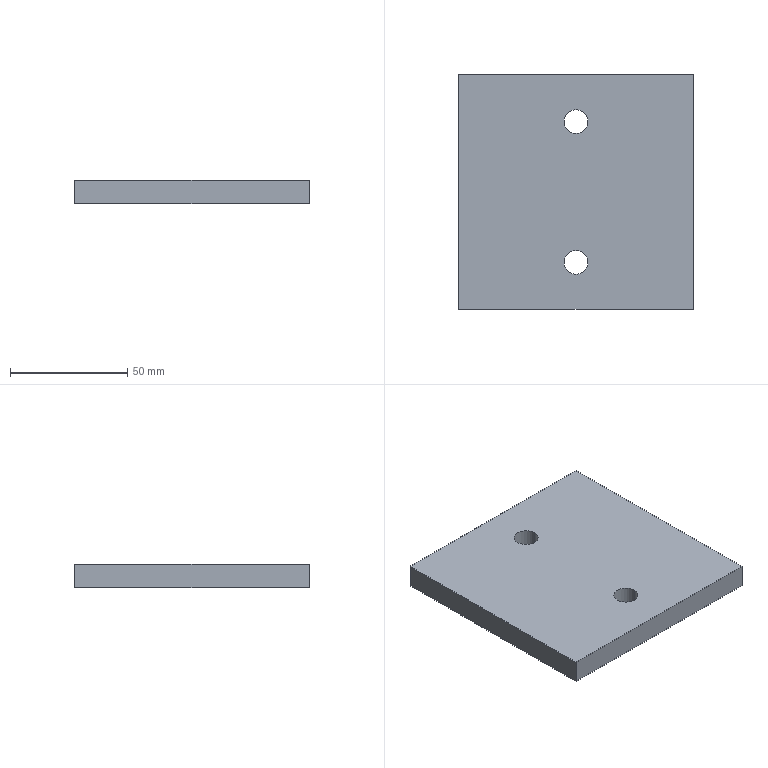Part | SolidWorks | features Extrusion 1, HoleWzd 1 | 1 solid | 10 faces | box 100 x 100 x 10 mm | volume 98366 mm3 | plane 6 | cylinder 4 | commonest cylinder face diameters 10.2 x4
STEP:
#1=CARTESIAN_POINT('',(5.1,30.,0.));
#2=VERTEX_POINT('',#1);
#3=CARTESIAN_POINT('',(-5.1,30.,0.));
#4=VERTEX_POINT('',#3);
#5=CARTESIAN_POINT('',(0.,30.,0.));
#6=DIRECTION('',(0.,0.,-1.));
#7=DIRECTION('',(-1.,0.,0.));
#8=AXIS2_PLACEMENT_3D('',#5,#6,#7);
#9=CIRCLE('',#8,5.1);
#10=EDGE_CURVE('',#2,#4,#9,.T.);
#11=ORIENTED_EDGE('',*,*,#10,.T.);
#12=CARTESIAN_POINT('',(-5.1,30.,10.));
#13=VERTEX_POINT('',#12);
#14=CARTESIAN_POINT('',(-5.1,30.,10.));
#15=DIRECTION('',(0.,0.,1.));
#16=VECTOR('',#15,1000.);
#17=LINE('',#14,#16);
#18=EDGE_CURVE('',#4,#13,#17,.T.);
#19=ORIENTED_EDGE('',*,*,#18,.T.);
#20=CARTESIAN_POINT('',(5.1,30.,10.));
#21=VERTEX_POINT('',#20);
#22=CARTESIAN_POINT('',(0.,30.,10.));
#23=DIRECTION('',(0.,0.,1.));
#24=DIRECTION('',(1.,0.,0.));
#25=AXIS2_PLACEMENT_3D('',#22,#23,#24);
#26=CIRCLE('',#25,5.1);
#27=EDGE_CURVE('',#13,#21,#26,.T.);
#28=ORIENTED_EDGE('',*,*,#27,.T.);
#29=CARTESIAN_POINT('',(5.1,30.,10.));
#30=DIRECTION('',(0.,0.,1.));
#31=VECTOR('',#30,1000.);
#32=LINE('',#29,#31);
#33=EDGE_CURVE('',#2,#21,#32,.T.);
#34=ORIENTED_EDGE('',*,*,#33,.F.);
#35=EDGE_LOOP('',(#11,#19,#28,#34));
#36=FACE_OUTER_BOUND('',#35,.T.);
#37=CARTESIAN_POINT('',(0.,30.,10.));
#38=DIRECTION('',(0.,0.,1.));
#39=DIRECTION('',(1.,0.,0.));
#40=AXIS2_PLACEMENT_3D('',#37,#38,#39);
#41=CYLINDRICAL_SURFACE('',#40,5.1);
#42=ADVANCED_FACE('',(#36),#41,.F.);
#43=CARTESIAN_POINT('',(5.1,-30.,0.));
#44=VERTEX_POINT('',#43);
#45=CARTESIAN_POINT('',(-5.1,-30.,0.));
#46=VERTEX_POINT('',#45);
#47=CARTESIAN_POINT('',(0.,-30.,0.));
#48=DIRECTION('',(0.,0.,-1.));
#49=DIRECTION('',(-1.,0.,0.));
#50=AXIS2_PLACEMENT_3D('',#47,#48,#49);
#51=CIRCLE('',#50,5.1);
#52=EDGE_CURVE('',#44,#46,#51,.T.);
#53=ORIENTED_EDGE('',*,*,#52,.T.);
#54=CARTESIAN_POINT('',(-5.1,-30.,10.));
#55=VERTEX_POINT('',#54);
#56=CARTESIAN_POINT('',(-5.1,-30.,10.));
#57=DIRECTION('',(0.,0.,1.));
#58=VECTOR('',#57,1000.);
#59=LINE('',#56,#58);
#60=EDGE_CURVE('',#46,#55,#59,.T.);
#61=ORIENTED_EDGE('',*,*,#60,.T.);
#62=CARTESIAN_POINT('',(5.1,-30.,10.));
#63=VERTEX_POINT('',#62);
#64=CARTESIAN_POINT('',(0.,-30.,10.));
#65=DIRECTION('',(0.,0.,1.));
#66=DIRECTION('',(1.,0.,0.));
#67=AXIS2_PLACEMENT_3D('',#64,#65,#66);
#68=CIRCLE('',#67,5.1);
#69=EDGE_CURVE('',#55,#63,#68,.T.);
#70=ORIENTED_EDGE('',*,*,#69,.T.);
#71=CARTESIAN_POINT('',(5.1,-30.,10.));
#72=DIRECTION('',(0.,0.,1.));
#73=VECTOR('',#72,1000.);
#74=LINE('',#71,#73);
#75=EDGE_CURVE('',#44,#63,#74,.T.);
#76=ORIENTED_EDGE('',*,*,#75,.F.);
#77=EDGE_LOOP('',(#53,#61,#70,#76));
#78=FACE_OUTER_BOUND('',#77,.T.);
#79=CARTESIAN_POINT('',(0.,-30.,10.));
#80=DIRECTION('',(0.,0.,1.));
#81=DIRECTION('',(1.,0.,0.));
#82=AXIS2_PLACEMENT_3D('',#79,#80,#81);
#83=CYLINDRICAL_SURFACE('',#82,5.1);
#84=ADVANCED_FACE('',(#78),#83,.F.);
#85=CARTESIAN_POINT('',(-50.,50.,0.));
#86=VERTEX_POINT('',#85);
#87=CARTESIAN_POINT('',(-50.,-50.,0.));
#88=VERTEX_POINT('',#87);
#89=CARTESIAN_POINT('',(-50.,50.,0.));
#90=DIRECTION('',(0.,-1.,0.));
#91=VECTOR('',#90,1000.);
#92=LINE('',#89,#91);
#93=EDGE_CURVE('',#86,#88,#92,.T.);
#94=ORIENTED_EDGE('',*,*,#93,.T.);
#95=CARTESIAN_POINT('',(-50.,-50.,10.));
#96=VERTEX_POINT('',#95);
#97=CARTESIAN_POINT('',(-50.,-50.,10.));
#98=DIRECTION('',(0.,0.,-1.));
#99=VECTOR('',#98,1000.);
#100=LINE('',#97,#99);
#101=EDGE_CURVE('',#96,#88,#100,.T.);
#102=ORIENTED_EDGE('',*,*,#101,.F.);
#103=CARTESIAN_POINT('',(-50.,50.,10.));
#104=VERTEX_POINT('',#103);
#105=CARTESIAN_POINT('',(-50.,50.,10.));
#106=DIRECTION('',(0.,-1.,0.));
#107=VECTOR('',#106,1000.);
#108=LINE('',#105,#107);
#109=EDGE_CURVE('',#104,#96,#108,.T.);
#110=ORIENTED_EDGE('',*,*,#109,.F.);
#111=CARTESIAN_POINT('',(-50.,50.,10.));
#112=DIRECTION('',(0.,0.,-1.));
#113=VECTOR('',#112,1000.);
#114=LINE('',#111,#113);
#115=EDGE_CURVE('',#104,#86,#114,.T.);
#116=ORIENTED_EDGE('',*,*,#115,.T.);
#117=EDGE_LOOP('',(#94,#102,#110,#116));
#118=FACE_OUTER_BOUND('',#117,.T.);
#119=CARTESIAN_POINT('',(-50.,50.,10.));
#120=DIRECTION('',(1.,0.,0.));
#121=DIRECTION('',(0.,1.,0.));
#122=AXIS2_PLACEMENT_3D('',#119,#120,#121);
#123=PLANE('',#122);
#124=ADVANCED_FACE('',(#118),#123,.F.);
#125=CARTESIAN_POINT('',(50.,-50.,0.));
#126=VERTEX_POINT('',#125);
#127=CARTESIAN_POINT('',(50.,-50.,0.));
#128=DIRECTION('',(1.,0.,0.));
#129=VECTOR('',#128,1000.);
#130=LINE('',#127,#129);
#131=EDGE_CURVE('',#88,#126,#130,.T.);
#132=ORIENTED_EDGE('',*,*,#131,.T.);
#133=CARTESIAN_POINT('',(50.,-50.,10.));
#134=VERTEX_POINT('',#133);
#135=CARTESIAN_POINT('',(50.,-50.,10.));
#136=DIRECTION('',(0.,0.,-1.));
#137=VECTOR('',#136,1000.);
#138=LINE('',#135,#137);
#139=EDGE_CURVE('',#134,#126,#138,.T.);
#140=ORIENTED_EDGE('',*,*,#139,.F.);
#141=CARTESIAN_POINT('',(50.,-50.,10.));
#142=DIRECTION('',(1.,0.,0.));
#143=VECTOR('',#142,1000.);
#144=LINE('',#141,#143);
#145=EDGE_CURVE('',#96,#134,#144,.T.);
#146=ORIENTED_EDGE('',*,*,#145,.F.);
#147=ORIENTED_EDGE('',*,*,#101,.T.);
#148=EDGE_LOOP('',(#132,#140,#146,#147));
#149=FACE_OUTER_BOUND('',#148,.T.);
#150=CARTESIAN_POINT('',(50.,-50.,10.));
#151=DIRECTION('',(0.,1.,0.));
#152=DIRECTION('',(-1.,0.,0.));
#153=AXIS2_PLACEMENT_3D('',#150,#151,#152);
#154=PLANE('',#153);
#155=ADVANCED_FACE('',(#149),#154,.F.);
#156=CARTESIAN_POINT('',(50.,50.,0.));
#157=VERTEX_POINT('',#156);
#158=CARTESIAN_POINT('',(50.,50.,0.));
#159=DIRECTION('',(0.,1.,0.));
#160=VECTOR('',#159,1000.);
#161=LINE('',#158,#160);
#162=EDGE_CURVE('',#126,#157,#161,.T.);
#163=ORIENTED_EDGE('',*,*,#162,.T.);
#164=CARTESIAN_POINT('',(50.,50.,10.));
#165=VERTEX_POINT('',#164);
#166=CARTESIAN_POINT('',(50.,50.,10.));
#167=DIRECTION('',(0.,0.,-1.));
#168=VECTOR('',#167,1000.);
#169=LINE('',#166,#168);
#170=EDGE_CURVE('',#165,#157,#169,.T.);
#171=ORIENTED_EDGE('',*,*,#170,.F.);
#172=CARTESIAN_POINT('',(50.,50.,10.));
#173=DIRECTION('',(0.,1.,0.));
#174=VECTOR('',#173,1000.);
#175=LINE('',#172,#174);
#176=EDGE_CURVE('',#134,#165,#175,.T.);
#177=ORIENTED_EDGE('',*,*,#176,.F.);
#178=ORIENTED_EDGE('',*,*,#139,.T.);
#179=EDGE_LOOP('',(#163,#171,#177,#178));
#180=FACE_OUTER_BOUND('',#179,.T.);
#181=CARTESIAN_POINT('',(50.,50.,10.));
#182=DIRECTION('',(-1.,0.,0.));
#183=DIRECTION('',(0.,-1.,0.));
#184=AXIS2_PLACEMENT_3D('',#181,#182,#183);
#185=PLANE('',#184);
#186=ADVANCED_FACE('',(#180),#185,.F.);
#187=CARTESIAN_POINT('',(50.,50.,0.));
#188=DIRECTION('',(-1.,0.,0.));
#189=VECTOR('',#188,1000.);
#190=LINE('',#187,#189);
#191=EDGE_CURVE('',#157,#86,#190,.T.);
#192=ORIENTED_EDGE('',*,*,#191,.T.);
#193=ORIENTED_EDGE('',*,*,#115,.F.);
#194=CARTESIAN_POINT('',(50.,50.,10.));
#195=DIRECTION('',(-1.,0.,0.));
#196=VECTOR('',#195,1000.);
#197=LINE('',#194,#196);
#198=EDGE_CURVE('',#165,#104,#197,.T.);
#199=ORIENTED_EDGE('',*,*,#198,.F.);
#200=ORIENTED_EDGE('',*,*,#170,.T.);
#201=EDGE_LOOP('',(#192,#193,#199,#200));
#202=FACE_OUTER_BOUND('',#201,.T.);
#203=CARTESIAN_POINT('',(50.,50.,10.));
#204=DIRECTION('',(0.,-1.,0.));
#205=DIRECTION('',(1.,0.,0.));
#206=AXIS2_PLACEMENT_3D('',#203,#204,#205);
#207=PLANE('',#206);
#208=ADVANCED_FACE('',(#202),#207,.F.);
#209=CARTESIAN_POINT('',(0.,30.,10.));
#210=DIRECTION('',(0.,0.,1.));
#211=DIRECTION('',(1.,0.,0.));
#212=AXIS2_PLACEMENT_3D('',#209,#210,#211);
#213=CIRCLE('',#212,5.1);
#214=EDGE_CURVE('',#21,#13,#213,.T.);
#215=ORIENTED_EDGE('',*,*,#214,.F.);
#216=ORIENTED_EDGE('',*,*,#27,.F.);
#217=EDGE_LOOP('',(#215,#216));
#218=FACE_BOUND('',#217,.T.);
#219=CARTESIAN_POINT('',(0.,-30.,10.));
#220=DIRECTION('',(0.,0.,1.));
#221=DIRECTION('',(1.,0.,0.));
#222=AXIS2_PLACEMENT_3D('',#219,#220,#221);
#223=CIRCLE('',#222,5.1);
#224=EDGE_CURVE('',#63,#55,#223,.T.);
#225=ORIENTED_EDGE('',*,*,#224,.F.);
#226=ORIENTED_EDGE('',*,*,#69,.F.);
#227=EDGE_LOOP('',(#225,#226));
#228=FACE_BOUND('',#227,.T.);
#229=ORIENTED_EDGE('',*,*,#109,.T.);
#230=ORIENTED_EDGE('',*,*,#145,.T.);
#231=ORIENTED_EDGE('',*,*,#176,.T.);
#232=ORIENTED_EDGE('',*,*,#198,.T.);
#233=EDGE_LOOP('',(#229,#230,#231,#232));
#234=FACE_OUTER_BOUND('',#233,.T.);
#235=CARTESIAN_POINT('',(0.,0.,10.));
#236=DIRECTION('',(0.,0.,-1.));
#237=DIRECTION('',(-1.,0.,0.));
#238=AXIS2_PLACEMENT_3D('',#235,#236,#237);
#239=PLANE('',#238);
#240=ADVANCED_FACE('',(#218,#228,#234),#239,.F.);
#241=ORIENTED_EDGE('',*,*,#10,.F.);
#242=CARTESIAN_POINT('',(0.,30.,0.));
#243=DIRECTION('',(0.,0.,-1.));
#244=DIRECTION('',(-1.,0.,0.));
#245=AXIS2_PLACEMENT_3D('',#242,#243,#244);
#246=CIRCLE('',#245,5.1);
#247=EDGE_CURVE('',#4,#2,#246,.T.);
#248=ORIENTED_EDGE('',*,*,#247,.F.);
#249=EDGE_LOOP('',(#241,#248));
#250=FACE_BOUND('',#249,.T.);
#251=ORIENTED_EDGE('',*,*,#52,.F.);
#252=CARTESIAN_POINT('',(0.,-30.,0.));
#253=DIRECTION('',(0.,0.,-1.));
#254=DIRECTION('',(-1.,0.,0.));
#255=AXIS2_PLACEMENT_3D('',#252,#253,#254);
#256=CIRCLE('',#255,5.1);
#257=EDGE_CURVE('',#46,#44,#256,.T.);
#258=ORIENTED_EDGE('',*,*,#257,.F.);
#259=EDGE_LOOP('',(#251,#258));
#260=FACE_BOUND('',#259,.T.);
#261=ORIENTED_EDGE('',*,*,#93,.F.);
#262=ORIENTED_EDGE('',*,*,#191,.F.);
#263=ORIENTED_EDGE('',*,*,#162,.F.);
#264=ORIENTED_EDGE('',*,*,#131,.F.);
#265=EDGE_LOOP('',(#261,#262,#263,#264));
#266=FACE_OUTER_BOUND('',#265,.T.);
#267=CARTESIAN_POINT('',(0.,0.,0.));
#268=DIRECTION('',(0.,0.,-1.));
#269=DIRECTION('',(-1.,0.,0.));
#270=AXIS2_PLACEMENT_3D('',#267,#268,#269);
#271=PLANE('',#270);
#272=ADVANCED_FACE('',(#250,#260,#266),#271,.T.);
#273=ORIENTED_EDGE('',*,*,#60,.F.);
#274=ORIENTED_EDGE('',*,*,#257,.T.);
#275=ORIENTED_EDGE('',*,*,#75,.T.);
#276=ORIENTED_EDGE('',*,*,#224,.T.);
#277=EDGE_LOOP('',(#273,#274,#275,#276));
#278=FACE_OUTER_BOUND('',#277,.T.);
#279=CARTESIAN_POINT('',(0.,-30.,10.));
#280=DIRECTION('',(0.,0.,1.));
#281=DIRECTION('',(1.,0.,0.));
#282=AXIS2_PLACEMENT_3D('',#279,#280,#281);
#283=CYLINDRICAL_SURFACE('',#282,5.1);
#284=ADVANCED_FACE('',(#278),#283,.F.);
#285=ORIENTED_EDGE('',*,*,#18,.F.);
#286=ORIENTED_EDGE('',*,*,#247,.T.);
#287=ORIENTED_EDGE('',*,*,#33,.T.);
#288=ORIENTED_EDGE('',*,*,#214,.T.);
#289=EDGE_LOOP('',(#285,#286,#287,#288));
#290=FACE_OUTER_BOUND('',#289,.T.);
#291=CARTESIAN_POINT('',(0.,30.,10.));
#292=DIRECTION('',(0.,0.,1.));
#293=DIRECTION('',(1.,0.,0.));
#294=AXIS2_PLACEMENT_3D('',#291,#292,#293);
#295=CYLINDRICAL_SURFACE('',#294,5.1);
#296=ADVANCED_FACE('',(#290),#295,.F.);
#297=CLOSED_SHELL('',(#42,#84,#124,#155,#186,#208,#240,#272,#284,#296));
#298=MANIFOLD_SOLID_BREP('',#297);
#299=CARTESIAN_POINT('',(0.,0.,0.));
#300=DIRECTION('',(0.,0.,1.));
#301=DIRECTION('',(1.,0.,0.));
#302=AXIS2_PLACEMENT_3D('',#299,#300,#301);
#303=(LENGTH_UNIT()NAMED_UNIT(*)SI_UNIT(.MILLI.,.METRE.));
#304=UNCERTAINTY_MEASURE_WITH_UNIT(LENGTH_MEASURE(0.00001),#303,'','');
#305=(NAMED_UNIT(*)PLANE_ANGLE_UNIT()SI_UNIT($,.RADIAN.));
#306=(NAMED_UNIT(*)SI_UNIT($,.STERADIAN.)SOLID_ANGLE_UNIT());
#307=(GEOMETRIC_REPRESENTATION_CONTEXT(3)GLOBAL_UNCERTAINTY_ASSIGNED_CONTEXT((#304))GLOBAL_UNIT_ASSIGNED_CONTEXT((#303,#305,#306))REPRESENTATION_CONTEXT('',''));
#308=ADVANCED_BREP_SHAPE_REPRESENTATION('',(#298,#302),#307);